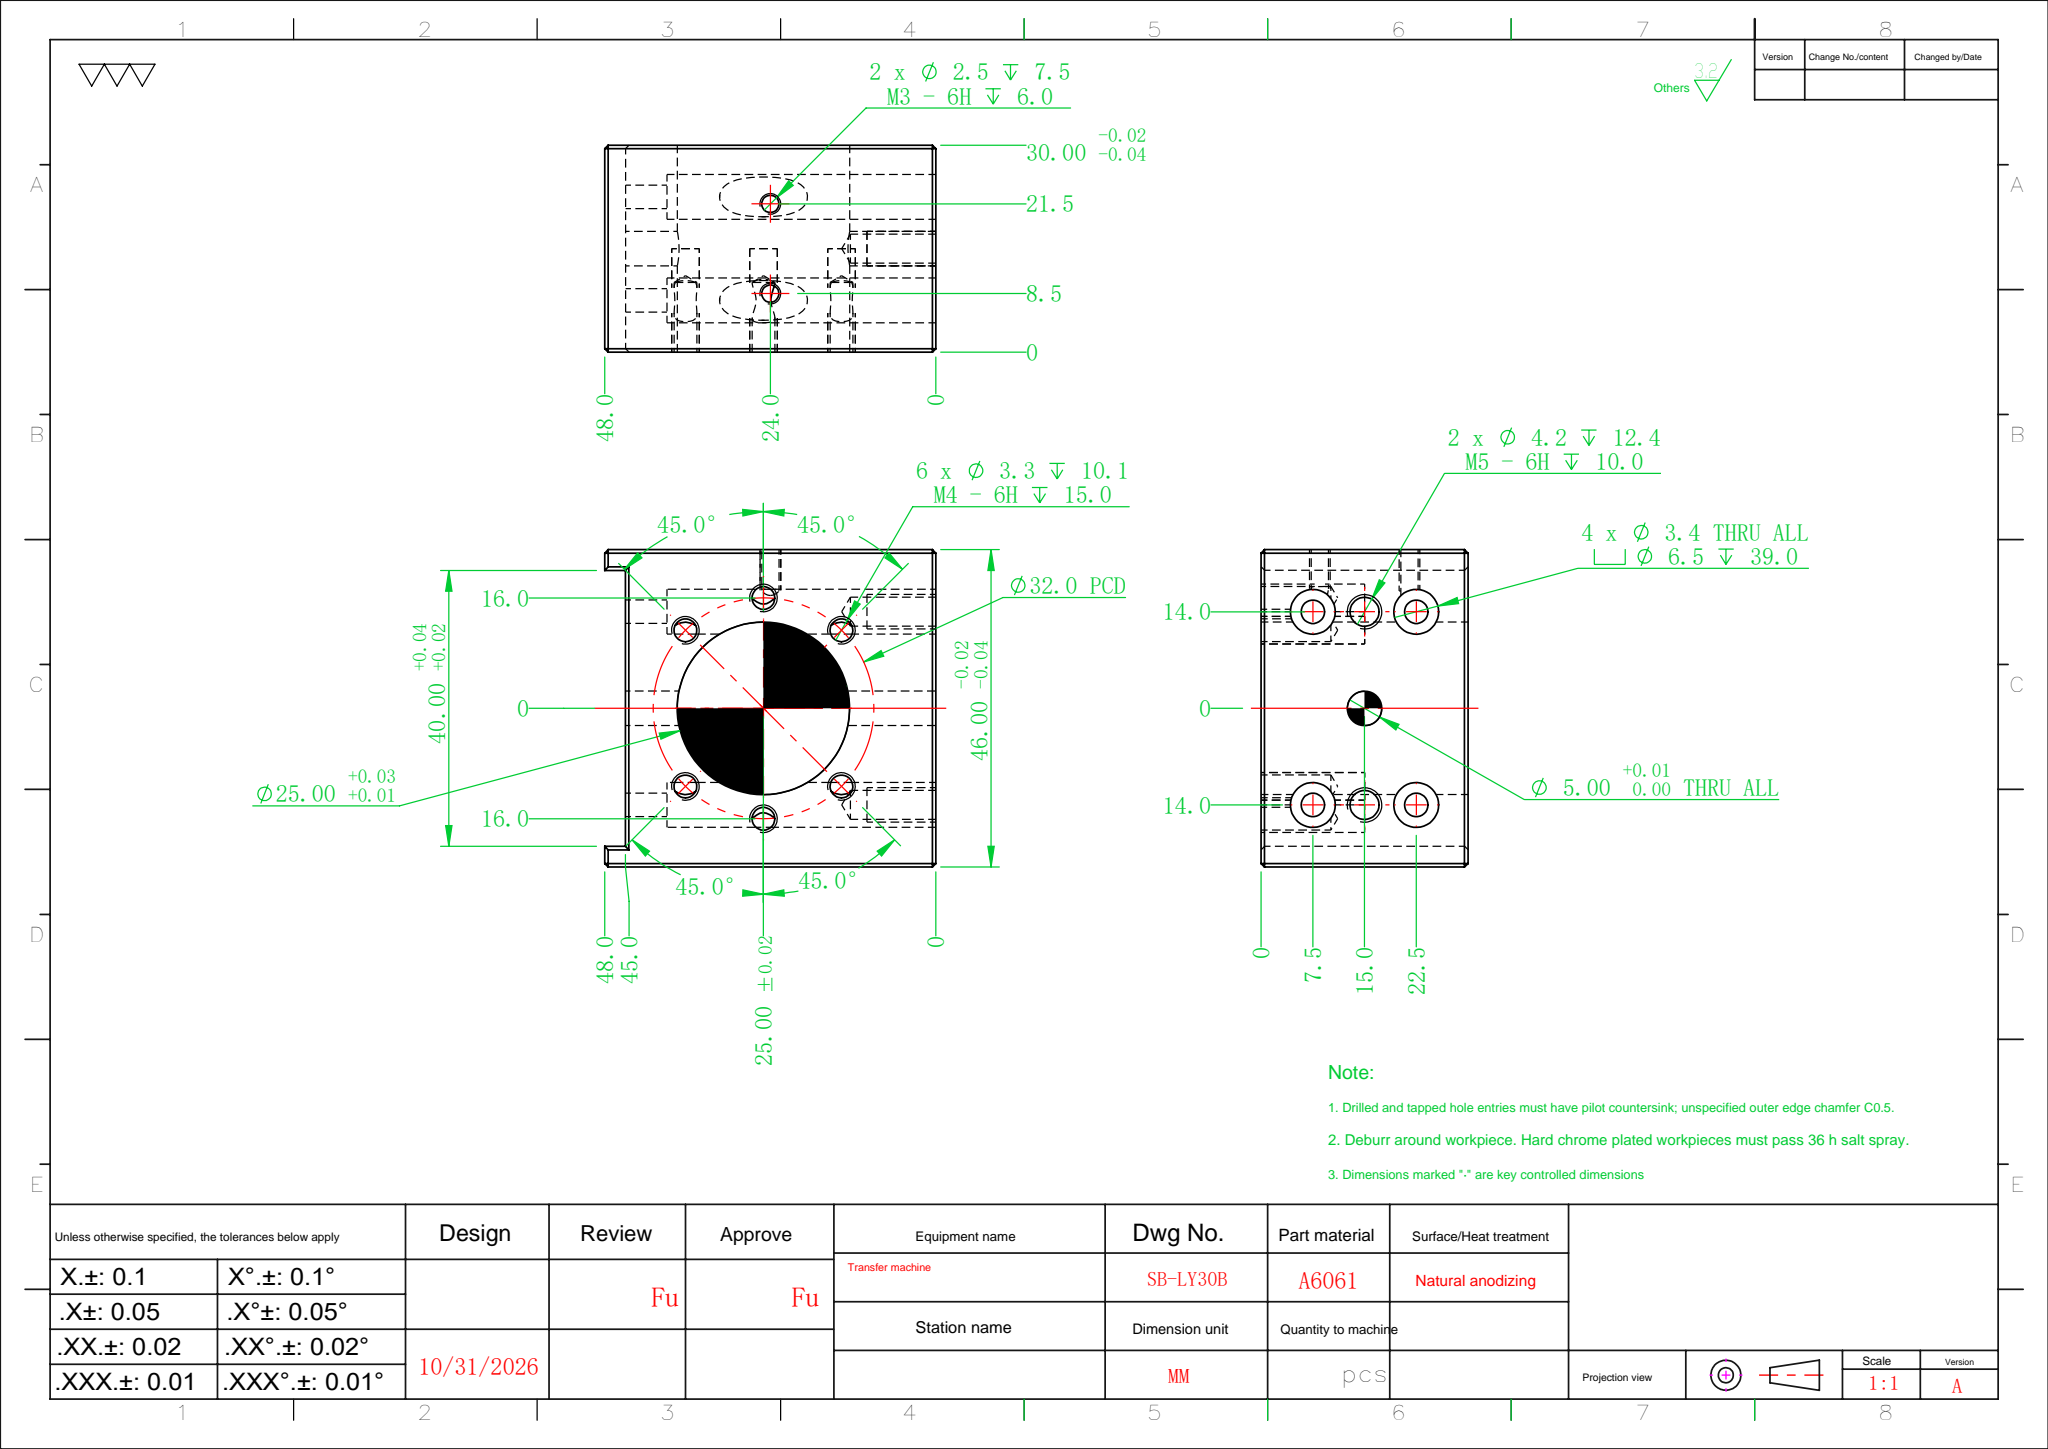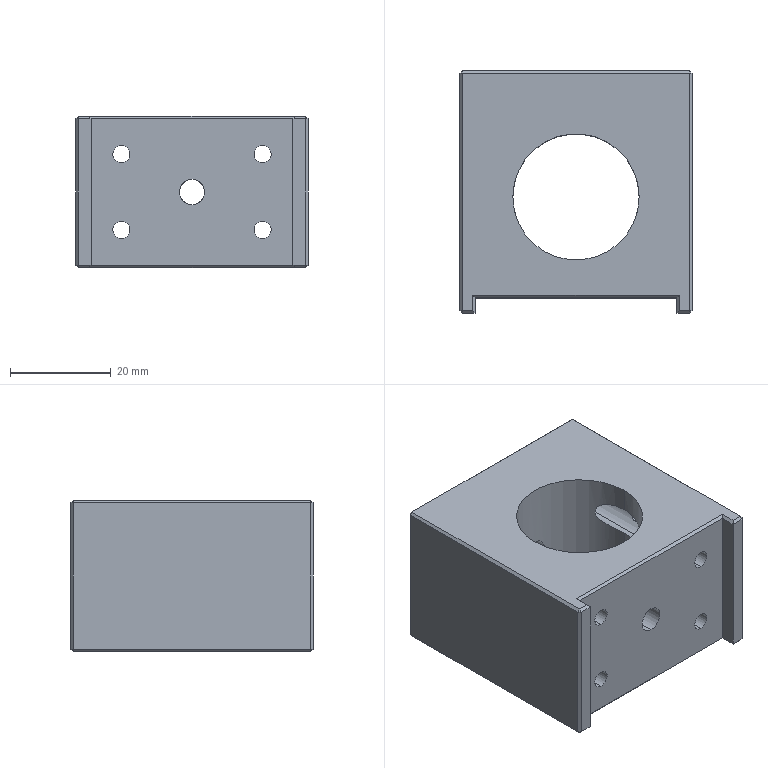Part | SolidWorks | features HoleWzd 5, Chamfer 1, Cut 1, Extrusion 1, ICE 1 | 1 solid | 101 faces | box 46 x 48 x 30 mm | volume 41518 mm3 | cylinder 43 | plane 42 | cone 16 | commonest cylinder face diameters 3.3 x13 3.4 x8 6.5 x8 2.5 x4 4.2 x4 5 x4